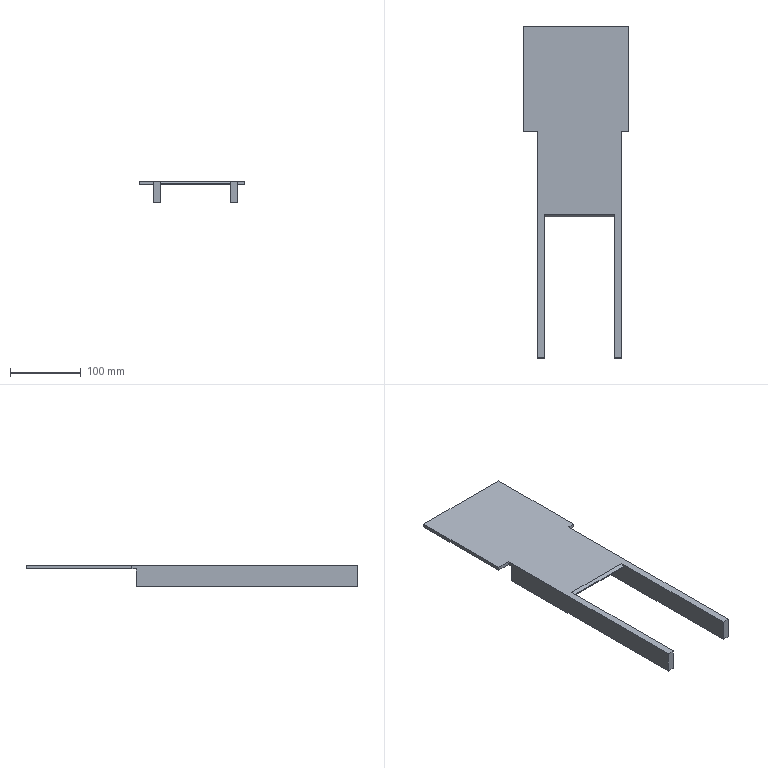Part | SolidWorks | features Chamfer 1, Extrusion 1, ICE 1 | 1 solid | 19 faces | box 150 x 470 x 30 mm | volume 353727 mm3 | plane 19
STEP:
#1=CARTESIAN_POINT('',(60.,40.,5.));
#2=VERTEX_POINT('',#1);
#3=CARTESIAN_POINT('',(60.,40.,0.));
#4=VERTEX_POINT('',#3);
#5=CARTESIAN_POINT('',(60.,40.,5.));
#6=DIRECTION('',(0.,0.,-1.));
#7=VECTOR('',#6,1000.);
#8=LINE('',#5,#7);
#9=EDGE_CURVE('',#2,#4,#8,.T.);
#10=ORIENTED_EDGE('',*,*,#9,.F.);
#11=CARTESIAN_POINT('',(60.,-280.,5.));
#12=VERTEX_POINT('',#11);
#13=CARTESIAN_POINT('',(60.,40.,5.));
#14=DIRECTION('',(0.,1.,0.));
#15=VECTOR('',#14,1000.);
#16=LINE('',#13,#15);
#17=EDGE_CURVE('',#12,#2,#16,.T.);
#18=ORIENTED_EDGE('',*,*,#17,.F.);
#19=CARTESIAN_POINT('',(60.,-280.,-25.));
#20=VERTEX_POINT('',#19);
#21=CARTESIAN_POINT('',(60.,-280.,-25.));
#22=DIRECTION('',(0.,0.,1.));
#23=VECTOR('',#22,1000.);
#24=LINE('',#21,#23);
#25=EDGE_CURVE('',#20,#12,#24,.T.);
#26=ORIENTED_EDGE('',*,*,#25,.F.);
#27=CARTESIAN_POINT('',(60.,5.758,-25.));
#28=VERTEX_POINT('',#27);
#29=CARTESIAN_POINT('',(60.,5.758,-25.));
#30=DIRECTION('',(0.,1.,0.));
#31=VECTOR('',#30,1000.);
#32=LINE('',#29,#31);
#33=EDGE_CURVE('',#20,#28,#32,.T.);
#34=ORIENTED_EDGE('',*,*,#33,.T.);
#35=CARTESIAN_POINT('',(60.,5.758,0.));
#36=VERTEX_POINT('',#35);
#37=CARTESIAN_POINT('',(60.,5.758,-25.));
#38=DIRECTION('',(0.,0.,1.));
#39=VECTOR('',#38,1000.);
#40=LINE('',#37,#39);
#41=EDGE_CURVE('',#28,#36,#40,.T.);
#42=ORIENTED_EDGE('',*,*,#41,.T.);
#43=CARTESIAN_POINT('',(60.,40.,0.));
#44=DIRECTION('',(0.,1.,0.));
#45=VECTOR('',#44,1000.);
#46=LINE('',#43,#45);
#47=EDGE_CURVE('',#36,#4,#46,.T.);
#48=ORIENTED_EDGE('',*,*,#47,.T.);
#49=EDGE_LOOP('',(#10,#18,#26,#34,#42,#48));
#50=FACE_OUTER_BOUND('',#49,.T.);
#51=CARTESIAN_POINT('',(60.,40.,5.));
#52=DIRECTION('',(-1.,0.,0.));
#53=DIRECTION('',(0.,-1.,0.));
#54=AXIS2_PLACEMENT_3D('',#51,#52,#53);
#55=PLANE('',#54);
#56=ADVANCED_FACE('',(#50),#55,.F.);
#57=CARTESIAN_POINT('',(70.,40.,0.));
#58=VERTEX_POINT('',#57);
#59=CARTESIAN_POINT('',(60.,40.,0.));
#60=DIRECTION('',(1.,0.,0.));
#61=VECTOR('',#60,1000.);
#62=LINE('',#59,#61);
#63=EDGE_CURVE('',#4,#58,#62,.T.);
#64=ORIENTED_EDGE('',*,*,#63,.T.);
#65=CARTESIAN_POINT('',(70.,40.,5.));
#66=VERTEX_POINT('',#65);
#67=CARTESIAN_POINT('',(70.,40.,5.));
#68=DIRECTION('',(0.,0.,-1.));
#69=VECTOR('',#68,1000.);
#70=LINE('',#67,#69);
#71=EDGE_CURVE('',#66,#58,#70,.T.);
#72=ORIENTED_EDGE('',*,*,#71,.F.);
#73=CARTESIAN_POINT('',(60.,40.,5.));
#74=DIRECTION('',(1.,0.,0.));
#75=VECTOR('',#74,1000.);
#76=LINE('',#73,#75);
#77=EDGE_CURVE('',#2,#66,#76,.T.);
#78=ORIENTED_EDGE('',*,*,#77,.F.);
#79=ORIENTED_EDGE('',*,*,#9,.T.);
#80=EDGE_LOOP('',(#64,#72,#78,#79));
#81=FACE_OUTER_BOUND('',#80,.T.);
#82=CARTESIAN_POINT('',(60.,40.,5.));
#83=DIRECTION('',(0.,1.,0.));
#84=DIRECTION('',(0.,0.,1.));
#85=AXIS2_PLACEMENT_3D('',#82,#83,#84);
#86=PLANE('',#85);
#87=ADVANCED_FACE('',(#81),#86,.F.);
#88=CARTESIAN_POINT('',(70.,190.,0.));
#89=VERTEX_POINT('',#88);
#90=CARTESIAN_POINT('',(70.,190.,0.));
#91=DIRECTION('',(0.,1.,0.));
#92=VECTOR('',#91,1000.);
#93=LINE('',#90,#92);
#94=EDGE_CURVE('',#58,#89,#93,.T.);
#95=ORIENTED_EDGE('',*,*,#94,.T.);
#96=CARTESIAN_POINT('',(70.,190.,5.));
#97=VERTEX_POINT('',#96);
#98=CARTESIAN_POINT('',(70.,190.,5.));
#99=DIRECTION('',(0.,0.,-1.));
#100=VECTOR('',#99,1000.);
#101=LINE('',#98,#100);
#102=EDGE_CURVE('',#97,#89,#101,.T.);
#103=ORIENTED_EDGE('',*,*,#102,.F.);
#104=CARTESIAN_POINT('',(70.,190.,5.));
#105=DIRECTION('',(0.,1.,0.));
#106=VECTOR('',#105,1000.);
#107=LINE('',#104,#106);
#108=EDGE_CURVE('',#66,#97,#107,.T.);
#109=ORIENTED_EDGE('',*,*,#108,.F.);
#110=ORIENTED_EDGE('',*,*,#71,.T.);
#111=EDGE_LOOP('',(#95,#103,#109,#110));
#112=FACE_OUTER_BOUND('',#111,.T.);
#113=CARTESIAN_POINT('',(70.,190.,5.));
#114=DIRECTION('',(-1.,0.,0.));
#115=DIRECTION('',(0.,-1.,0.));
#116=AXIS2_PLACEMENT_3D('',#113,#114,#115);
#117=PLANE('',#116);
#118=ADVANCED_FACE('',(#112),#117,.F.);
#119=CARTESIAN_POINT('',(-80.,190.,0.));
#120=VERTEX_POINT('',#119);
#121=CARTESIAN_POINT('',(-80.,190.,0.));
#122=DIRECTION('',(-1.,0.,0.));
#123=VECTOR('',#122,1000.);
#124=LINE('',#121,#123);
#125=EDGE_CURVE('',#89,#120,#124,.T.);
#126=ORIENTED_EDGE('',*,*,#125,.T.);
#127=CARTESIAN_POINT('',(-80.,190.,5.));
#128=VERTEX_POINT('',#127);
#129=CARTESIAN_POINT('',(-80.,190.,5.));
#130=DIRECTION('',(0.,0.,-1.));
#131=VECTOR('',#130,1000.);
#132=LINE('',#129,#131);
#133=EDGE_CURVE('',#128,#120,#132,.T.);
#134=ORIENTED_EDGE('',*,*,#133,.F.);
#135=CARTESIAN_POINT('',(-80.,190.,5.));
#136=DIRECTION('',(-1.,0.,0.));
#137=VECTOR('',#136,1000.);
#138=LINE('',#135,#137);
#139=EDGE_CURVE('',#97,#128,#138,.T.);
#140=ORIENTED_EDGE('',*,*,#139,.F.);
#141=ORIENTED_EDGE('',*,*,#102,.T.);
#142=EDGE_LOOP('',(#126,#134,#140,#141));
#143=FACE_OUTER_BOUND('',#142,.T.);
#144=CARTESIAN_POINT('',(-80.,190.,5.));
#145=DIRECTION('',(0.,-1.,0.));
#146=DIRECTION('',(0.,0.,-1.));
#147=AXIS2_PLACEMENT_3D('',#144,#145,#146);
#148=PLANE('',#147);
#149=ADVANCED_FACE('',(#143),#148,.F.);
#150=CARTESIAN_POINT('',(-80.,40.,0.));
#151=VERTEX_POINT('',#150);
#152=CARTESIAN_POINT('',(-80.,190.,0.));
#153=DIRECTION('',(0.,-1.,0.));
#154=VECTOR('',#153,1000.);
#155=LINE('',#152,#154);
#156=EDGE_CURVE('',#120,#151,#155,.T.);
#157=ORIENTED_EDGE('',*,*,#156,.T.);
#158=CARTESIAN_POINT('',(-80.,40.,5.));
#159=VERTEX_POINT('',#158);
#160=CARTESIAN_POINT('',(-80.,40.,5.));
#161=DIRECTION('',(0.,0.,-1.));
#162=VECTOR('',#161,1000.);
#163=LINE('',#160,#162);
#164=EDGE_CURVE('',#159,#151,#163,.T.);
#165=ORIENTED_EDGE('',*,*,#164,.F.);
#166=CARTESIAN_POINT('',(-80.,190.,5.));
#167=DIRECTION('',(0.,-1.,0.));
#168=VECTOR('',#167,1000.);
#169=LINE('',#166,#168);
#170=EDGE_CURVE('',#128,#159,#169,.T.);
#171=ORIENTED_EDGE('',*,*,#170,.F.);
#172=ORIENTED_EDGE('',*,*,#133,.T.);
#173=EDGE_LOOP('',(#157,#165,#171,#172));
#174=FACE_OUTER_BOUND('',#173,.T.);
#175=CARTESIAN_POINT('',(-80.,190.,5.));
#176=DIRECTION('',(1.,0.,0.));
#177=DIRECTION('',(0.,1.,0.));
#178=AXIS2_PLACEMENT_3D('',#175,#176,#177);
#179=PLANE('',#178);
#180=ADVANCED_FACE('',(#174),#179,.F.);
#181=CARTESIAN_POINT('',(-60.,40.,0.));
#182=VERTEX_POINT('',#181);
#183=CARTESIAN_POINT('',(-80.,40.,0.));
#184=DIRECTION('',(1.,0.,0.));
#185=VECTOR('',#184,1000.);
#186=LINE('',#183,#185);
#187=EDGE_CURVE('',#151,#182,#186,.T.);
#188=ORIENTED_EDGE('',*,*,#187,.T.);
#189=CARTESIAN_POINT('',(-60.,40.,5.));
#190=VERTEX_POINT('',#189);
#191=CARTESIAN_POINT('',(-60.,40.,5.));
#192=DIRECTION('',(0.,0.,-1.));
#193=VECTOR('',#192,1000.);
#194=LINE('',#191,#193);
#195=EDGE_CURVE('',#190,#182,#194,.T.);
#196=ORIENTED_EDGE('',*,*,#195,.F.);
#197=CARTESIAN_POINT('',(-80.,40.,5.));
#198=DIRECTION('',(1.,0.,0.));
#199=VECTOR('',#198,1000.);
#200=LINE('',#197,#199);
#201=EDGE_CURVE('',#159,#190,#200,.T.);
#202=ORIENTED_EDGE('',*,*,#201,.F.);
#203=ORIENTED_EDGE('',*,*,#164,.T.);
#204=EDGE_LOOP('',(#188,#196,#202,#203));
#205=FACE_OUTER_BOUND('',#204,.T.);
#206=CARTESIAN_POINT('',(-80.,40.,5.));
#207=DIRECTION('',(0.,1.,0.));
#208=DIRECTION('',(0.,0.,1.));
#209=AXIS2_PLACEMENT_3D('',#206,#207,#208);
#210=PLANE('',#209);
#211=ADVANCED_FACE('',(#205),#210,.F.);
#212=CARTESIAN_POINT('',(-60.,33.599,0.));
#213=VERTEX_POINT('',#212);
#214=CARTESIAN_POINT('',(-60.,40.,0.));
#215=DIRECTION('',(0.,-1.,0.));
#216=VECTOR('',#215,1000.);
#217=LINE('',#214,#216);
#218=EDGE_CURVE('',#182,#213,#217,.T.);
#219=ORIENTED_EDGE('',*,*,#218,.T.);
#220=CARTESIAN_POINT('',(-60.,33.599,-25.));
#221=VERTEX_POINT('',#220);
#222=CARTESIAN_POINT('',(-60.,33.599,-25.));
#223=DIRECTION('',(0.,0.,1.));
#224=VECTOR('',#223,1000.);
#225=LINE('',#222,#224);
#226=EDGE_CURVE('',#221,#213,#225,.T.);
#227=ORIENTED_EDGE('',*,*,#226,.F.);
#228=CARTESIAN_POINT('',(-60.,-280.,-25.));
#229=VERTEX_POINT('',#228);
#230=CARTESIAN_POINT('',(-60.,33.599,-25.));
#231=DIRECTION('',(0.,-1.,0.));
#232=VECTOR('',#231,1000.);
#233=LINE('',#230,#232);
#234=EDGE_CURVE('',#221,#229,#233,.T.);
#235=ORIENTED_EDGE('',*,*,#234,.T.);
#236=CARTESIAN_POINT('',(-60.,-280.,5.));
#237=VERTEX_POINT('',#236);
#238=CARTESIAN_POINT('',(-60.,-280.,-25.));
#239=DIRECTION('',(0.,0.,1.));
#240=VECTOR('',#239,1000.);
#241=LINE('',#238,#240);
#242=EDGE_CURVE('',#229,#237,#241,.T.);
#243=ORIENTED_EDGE('',*,*,#242,.T.);
#244=CARTESIAN_POINT('',(-60.,40.,5.));
#245=DIRECTION('',(0.,-1.,0.));
#246=VECTOR('',#245,1000.);
#247=LINE('',#244,#246);
#248=EDGE_CURVE('',#190,#237,#247,.T.);
#249=ORIENTED_EDGE('',*,*,#248,.F.);
#250=ORIENTED_EDGE('',*,*,#195,.T.);
#251=EDGE_LOOP('',(#219,#227,#235,#243,#249,#250));
#252=FACE_OUTER_BOUND('',#251,.T.);
#253=CARTESIAN_POINT('',(-60.,40.,5.));
#254=DIRECTION('',(1.,0.,0.));
#255=DIRECTION('',(0.,1.,0.));
#256=AXIS2_PLACEMENT_3D('',#253,#254,#255);
#257=PLANE('',#256);
#258=ADVANCED_FACE('',(#252),#257,.F.);
#259=CARTESIAN_POINT('',(50.,-80.,0.));
#260=VERTEX_POINT('',#259);
#261=CARTESIAN_POINT('',(50.,-80.,1.5));
#262=VERTEX_POINT('',#261);
#263=CARTESIAN_POINT('',(50.,-80.,5.));
#264=DIRECTION('',(0.,0.,1.));
#265=VECTOR('',#264,1000.);
#266=LINE('',#263,#265);
#267=EDGE_CURVE('',#260,#262,#266,.T.);
#268=ORIENTED_EDGE('',*,*,#267,.T.);
#269=CARTESIAN_POINT('',(-50.,-80.,1.5));
#270=VERTEX_POINT('',#269);
#271=CARTESIAN_POINT('',(-50.,-80.,1.5));
#272=DIRECTION('',(-1.,0.,0.));
#273=VECTOR('',#272,1000.);
#274=LINE('',#271,#273);
#275=EDGE_CURVE('',#262,#270,#274,.T.);
#276=ORIENTED_EDGE('',*,*,#275,.T.);
#277=CARTESIAN_POINT('',(-50.,-80.,0.));
#278=VERTEX_POINT('',#277);
#279=CARTESIAN_POINT('',(-50.,-80.,5.));
#280=DIRECTION('',(0.,0.,-1.));
#281=VECTOR('',#280,1000.);
#282=LINE('',#279,#281);
#283=EDGE_CURVE('',#270,#278,#282,.T.);
#284=ORIENTED_EDGE('',*,*,#283,.T.);
#285=CARTESIAN_POINT('',(-60.,-80.,0.));
#286=DIRECTION('',(1.,0.,0.));
#287=VECTOR('',#286,1000.);
#288=LINE('',#285,#287);
#289=EDGE_CURVE('',#278,#260,#288,.T.);
#290=ORIENTED_EDGE('',*,*,#289,.T.);
#291=EDGE_LOOP('',(#268,#276,#284,#290));
#292=FACE_OUTER_BOUND('',#291,.T.);
#293=CARTESIAN_POINT('',(-60.,-80.,5.));
#294=DIRECTION('',(0.,1.,0.));
#295=DIRECTION('',(0.,0.,1.));
#296=AXIS2_PLACEMENT_3D('',#293,#294,#295);
#297=PLANE('',#296);
#298=ADVANCED_FACE('',(#292),#297,.F.);
#299=CARTESIAN_POINT('',(-50.,-76.5,5.));
#300=VERTEX_POINT('',#299);
#301=CARTESIAN_POINT('',(50.,-76.5,5.));
#302=VERTEX_POINT('',#301);
#303=CARTESIAN_POINT('',(50.,-76.5,5.));
#304=DIRECTION('',(1.,0.,0.));
#305=VECTOR('',#304,1000.);
#306=LINE('',#303,#305);
#307=EDGE_CURVE('',#300,#302,#306,.T.);
#308=ORIENTED_EDGE('',*,*,#307,.T.);
#309=CARTESIAN_POINT('',(50.,-280.,5.));
#310=VERTEX_POINT('',#309);
#311=CARTESIAN_POINT('',(50.,5.758,5.));
#312=DIRECTION('',(0.,-1.,0.));
#313=VECTOR('',#312,1000.);
#314=LINE('',#311,#313);
#315=EDGE_CURVE('',#302,#310,#314,.T.);
#316=ORIENTED_EDGE('',*,*,#315,.T.);
#317=CARTESIAN_POINT('',(60.,-280.,5.));
#318=DIRECTION('',(1.,0.,0.));
#319=VECTOR('',#318,1000.);
#320=LINE('',#317,#319);
#321=EDGE_CURVE('',#310,#12,#320,.T.);
#322=ORIENTED_EDGE('',*,*,#321,.T.);
#323=ORIENTED_EDGE('',*,*,#17,.T.);
#324=ORIENTED_EDGE('',*,*,#77,.T.);
#325=ORIENTED_EDGE('',*,*,#108,.T.);
#326=ORIENTED_EDGE('',*,*,#139,.T.);
#327=ORIENTED_EDGE('',*,*,#170,.T.);
#328=ORIENTED_EDGE('',*,*,#201,.T.);
#329=ORIENTED_EDGE('',*,*,#248,.T.);
#330=CARTESIAN_POINT('',(-50.,-280.,5.));
#331=VERTEX_POINT('',#330);
#332=CARTESIAN_POINT('',(-60.,-280.,5.));
#333=DIRECTION('',(1.,0.,0.));
#334=VECTOR('',#333,1000.);
#335=LINE('',#332,#334);
#336=EDGE_CURVE('',#237,#331,#335,.T.);
#337=ORIENTED_EDGE('',*,*,#336,.T.);
#338=CARTESIAN_POINT('',(-50.,33.599,5.));
#339=DIRECTION('',(0.,1.,0.));
#340=VECTOR('',#339,1000.);
#341=LINE('',#338,#340);
#342=EDGE_CURVE('',#331,#300,#341,.T.);
#343=ORIENTED_EDGE('',*,*,#342,.T.);
#344=EDGE_LOOP('',(#308,#316,#322,#323,#324,#325,#326,#327,#328,#329,#337,#343));
#345=FACE_OUTER_BOUND('',#344,.T.);
#346=CARTESIAN_POINT('',(0.,0.,5.));
#347=DIRECTION('',(0.,0.,1.));
#348=DIRECTION('',(1.,0.,0.));
#349=AXIS2_PLACEMENT_3D('',#346,#347,#348);
#350=PLANE('',#349);
#351=ADVANCED_FACE('',(#345),#350,.T.);
#352=CARTESIAN_POINT('',(-50.,33.599,0.));
#353=VERTEX_POINT('',#352);
#354=CARTESIAN_POINT('',(-50.,0.,0.));
#355=DIRECTION('',(0.,1.,0.));
#356=VECTOR('',#355,1000.);
#357=LINE('',#354,#356);
#358=EDGE_CURVE('',#278,#353,#357,.T.);
#359=ORIENTED_EDGE('',*,*,#358,.T.);
#360=CARTESIAN_POINT('',(0.,33.599,0.));
#361=DIRECTION('',(-1.,0.,0.));
#362=VECTOR('',#361,1000.);
#363=LINE('',#360,#362);
#364=EDGE_CURVE('',#353,#213,#363,.T.);
#365=ORIENTED_EDGE('',*,*,#364,.T.);
#366=ORIENTED_EDGE('',*,*,#218,.F.);
#367=ORIENTED_EDGE('',*,*,#187,.F.);
#368=ORIENTED_EDGE('',*,*,#156,.F.);
#369=ORIENTED_EDGE('',*,*,#125,.F.);
#370=ORIENTED_EDGE('',*,*,#94,.F.);
#371=ORIENTED_EDGE('',*,*,#63,.F.);
#372=ORIENTED_EDGE('',*,*,#47,.F.);
#373=CARTESIAN_POINT('',(50.,5.758,0.));
#374=VERTEX_POINT('',#373);
#375=CARTESIAN_POINT('',(0.,5.758,0.));
#376=DIRECTION('',(-1.,0.,0.));
#377=VECTOR('',#376,1000.);
#378=LINE('',#375,#377);
#379=EDGE_CURVE('',#36,#374,#378,.T.);
#380=ORIENTED_EDGE('',*,*,#379,.T.);
#381=CARTESIAN_POINT('',(50.,0.,0.));
#382=DIRECTION('',(0.,-1.,0.));
#383=VECTOR('',#382,1000.);
#384=LINE('',#381,#383);
#385=EDGE_CURVE('',#374,#260,#384,.T.);
#386=ORIENTED_EDGE('',*,*,#385,.T.);
#387=ORIENTED_EDGE('',*,*,#289,.F.);
#388=EDGE_LOOP('',(#359,#365,#366,#367,#368,#369,#370,#371,#372,#380,#386,#387));
#389=FACE_OUTER_BOUND('',#388,.T.);
#390=CARTESIAN_POINT('',(0.,0.,0.));
#391=DIRECTION('',(0.,0.,1.));
#392=DIRECTION('',(1.,0.,0.));
#393=AXIS2_PLACEMENT_3D('',#390,#391,#392);
#394=PLANE('',#393);
#395=ADVANCED_FACE('',(#389),#394,.F.);
#396=ORIENTED_EDGE('',*,*,#267,.F.);
#397=ORIENTED_EDGE('',*,*,#385,.F.);
#398=CARTESIAN_POINT('',(50.,5.758,-25.));
#399=VERTEX_POINT('',#398);
#400=CARTESIAN_POINT('',(50.,5.758,-25.));
#401=DIRECTION('',(0.,0.,1.));
#402=VECTOR('',#401,1000.);
#403=LINE('',#400,#402);
#404=EDGE_CURVE('',#399,#374,#403,.T.);
#405=ORIENTED_EDGE('',*,*,#404,.F.);
#406=CARTESIAN_POINT('',(50.,-280.,-25.));
#407=VERTEX_POINT('',#406);
#408=CARTESIAN_POINT('',(50.,5.758,-25.));
#409=DIRECTION('',(0.,-1.,0.));
#410=VECTOR('',#409,1000.);
#411=LINE('',#408,#410);
#412=EDGE_CURVE('',#399,#407,#411,.T.);
#413=ORIENTED_EDGE('',*,*,#412,.T.);
#414=CARTESIAN_POINT('',(50.,-280.,-25.));
#415=DIRECTION('',(0.,0.,1.));
#416=VECTOR('',#415,1000.);
#417=LINE('',#414,#416);
#418=EDGE_CURVE('',#407,#310,#417,.T.);
#419=ORIENTED_EDGE('',*,*,#418,.T.);
#420=ORIENTED_EDGE('',*,*,#315,.F.);
#421=CARTESIAN_POINT('',(50.,-76.5,5.));
#422=DIRECTION('',(0.,-0.7071,-0.7071));
#423=VECTOR('',#422,1000.);
#424=LINE('',#421,#423);
#425=EDGE_CURVE('',#302,#262,#424,.T.);
#426=ORIENTED_EDGE('',*,*,#425,.T.);
#427=EDGE_LOOP('',(#396,#397,#405,#413,#419,#420,#426));
#428=FACE_OUTER_BOUND('',#427,.T.);
#429=CARTESIAN_POINT('',(50.,5.758,-25.));
#430=DIRECTION('',(-1.,0.,0.));
#431=DIRECTION('',(0.,-1.,0.));
#432=AXIS2_PLACEMENT_3D('',#429,#430,#431);
#433=PLANE('',#432);
#434=ADVANCED_FACE('',(#428),#433,.T.);
#435=ORIENTED_EDGE('',*,*,#379,.F.);
#436=ORIENTED_EDGE('',*,*,#41,.F.);
#437=CARTESIAN_POINT('',(60.,5.758,-25.));
#438=DIRECTION('',(-1.,0.,0.));
#439=VECTOR('',#438,1000.);
#440=LINE('',#437,#439);
#441=EDGE_CURVE('',#28,#399,#440,.T.);
#442=ORIENTED_EDGE('',*,*,#441,.T.);
#443=ORIENTED_EDGE('',*,*,#404,.T.);
#444=EDGE_LOOP('',(#435,#436,#442,#443));
#445=FACE_OUTER_BOUND('',#444,.T.);
#446=CARTESIAN_POINT('',(60.,5.758,-25.));
#447=DIRECTION('',(0.,1.,0.));
#448=DIRECTION('',(-1.,0.,0.));
#449=AXIS2_PLACEMENT_3D('',#446,#447,#448);
#450=PLANE('',#449);
#451=ADVANCED_FACE('',(#445),#450,.T.);
#452=ORIENTED_EDGE('',*,*,#321,.F.);
#453=ORIENTED_EDGE('',*,*,#418,.F.);
#454=CARTESIAN_POINT('',(60.,-280.,-25.));
#455=DIRECTION('',(1.,0.,0.));
#456=VECTOR('',#455,1000.);
#457=LINE('',#454,#456);
#458=EDGE_CURVE('',#407,#20,#457,.T.);
#459=ORIENTED_EDGE('',*,*,#458,.T.);
#460=ORIENTED_EDGE('',*,*,#25,.T.);
#461=EDGE_LOOP('',(#452,#453,#459,#460));
#462=FACE_OUTER_BOUND('',#461,.T.);
#463=CARTESIAN_POINT('',(60.,-280.,-25.));
#464=DIRECTION('',(0.,-1.,0.));
#465=DIRECTION('',(0.,0.,-1.));
#466=AXIS2_PLACEMENT_3D('',#463,#464,#465);
#467=PLANE('',#466);
#468=ADVANCED_FACE('',(#462),#467,.T.);
#469=ORIENTED_EDGE('',*,*,#33,.F.);
#470=ORIENTED_EDGE('',*,*,#458,.F.);
#471=ORIENTED_EDGE('',*,*,#412,.F.);
#472=ORIENTED_EDGE('',*,*,#441,.F.);
#473=EDGE_LOOP('',(#469,#470,#471,#472));
#474=FACE_OUTER_BOUND('',#473,.T.);
#475=CARTESIAN_POINT('',(0.,0.,-25.));
#476=DIRECTION('',(0.,0.,-1.));
#477=DIRECTION('',(-1.,0.,0.));
#478=AXIS2_PLACEMENT_3D('',#475,#476,#477);
#479=PLANE('',#478);
#480=ADVANCED_FACE('',(#474),#479,.T.);
#481=ORIENTED_EDGE('',*,*,#364,.F.);
#482=CARTESIAN_POINT('',(-50.,33.599,-25.));
#483=VERTEX_POINT('',#482);
#484=CARTESIAN_POINT('',(-50.,33.599,-25.));
#485=DIRECTION('',(0.,0.,1.));
#486=VECTOR('',#485,1000.);
#487=LINE('',#484,#486);
#488=EDGE_CURVE('',#483,#353,#487,.T.);
#489=ORIENTED_EDGE('',*,*,#488,.F.);
#490=CARTESIAN_POINT('',(-60.,33.599,-25.));
#491=DIRECTION('',(-1.,0.,0.));
#492=VECTOR('',#491,1000.);
#493=LINE('',#490,#492);
#494=EDGE_CURVE('',#483,#221,#493,.T.);
#495=ORIENTED_EDGE('',*,*,#494,.T.);
#496=ORIENTED_EDGE('',*,*,#226,.T.);
#497=EDGE_LOOP('',(#481,#489,#495,#496));
#498=FACE_OUTER_BOUND('',#497,.T.);
#499=CARTESIAN_POINT('',(-60.,33.599,-25.));
#500=DIRECTION('',(0.,1.,0.));
#501=DIRECTION('',(0.,0.,1.));
#502=AXIS2_PLACEMENT_3D('',#499,#500,#501);
#503=PLANE('',#502);
#504=ADVANCED_FACE('',(#498),#503,.T.);
#505=ORIENTED_EDGE('',*,*,#283,.F.);
#506=CARTESIAN_POINT('',(-50.,-76.5,5.));
#507=DIRECTION('',(0.,0.7071,0.7071));
#508=VECTOR('',#507,1000.);
#509=LINE('',#506,#508);
#510=EDGE_CURVE('',#270,#300,#509,.T.);
#511=ORIENTED_EDGE('',*,*,#510,.T.);
#512=ORIENTED_EDGE('',*,*,#342,.F.);
#513=CARTESIAN_POINT('',(-50.,-280.,-25.));
#514=VERTEX_POINT('',#513);
#515=CARTESIAN_POINT('',(-50.,-280.,-25.));
#516=DIRECTION('',(0.,0.,1.));
#517=VECTOR('',#516,1000.);
#518=LINE('',#515,#517);
#519=EDGE_CURVE('',#514,#331,#518,.T.);
#520=ORIENTED_EDGE('',*,*,#519,.F.);
#521=CARTESIAN_POINT('',(-50.,33.599,-25.));
#522=DIRECTION('',(0.,1.,0.));
#523=VECTOR('',#522,1000.);
#524=LINE('',#521,#523);
#525=EDGE_CURVE('',#514,#483,#524,.T.);
#526=ORIENTED_EDGE('',*,*,#525,.T.);
#527=ORIENTED_EDGE('',*,*,#488,.T.);
#528=ORIENTED_EDGE('',*,*,#358,.F.);
#529=EDGE_LOOP('',(#505,#511,#512,#520,#526,#527,#528));
#530=FACE_OUTER_BOUND('',#529,.T.);
#531=CARTESIAN_POINT('',(-50.,33.599,-25.));
#532=DIRECTION('',(1.,0.,0.));
#533=DIRECTION('',(0.,1.,0.));
#534=AXIS2_PLACEMENT_3D('',#531,#532,#533);
#535=PLANE('',#534);
#536=ADVANCED_FACE('',(#530),#535,.T.);
#537=ORIENTED_EDGE('',*,*,#336,.F.);
#538=ORIENTED_EDGE('',*,*,#242,.F.);
#539=CARTESIAN_POINT('',(-60.,-280.,-25.));
#540=DIRECTION('',(1.,0.,0.));
#541=VECTOR('',#540,1000.);
#542=LINE('',#539,#541);
#543=EDGE_CURVE('',#229,#514,#542,.T.);
#544=ORIENTED_EDGE('',*,*,#543,.T.);
#545=ORIENTED_EDGE('',*,*,#519,.T.);
#546=EDGE_LOOP('',(#537,#538,#544,#545));
#547=FACE_OUTER_BOUND('',#546,.T.);
#548=CARTESIAN_POINT('',(-60.,-280.,-25.));
#549=DIRECTION('',(0.,-1.,0.));
#550=DIRECTION('',(0.,0.,-1.));
#551=AXIS2_PLACEMENT_3D('',#548,#549,#550);
#552=PLANE('',#551);
#553=ADVANCED_FACE('',(#547),#552,.T.);
#554=ORIENTED_EDGE('',*,*,#234,.F.);
#555=ORIENTED_EDGE('',*,*,#494,.F.);
#556=ORIENTED_EDGE('',*,*,#525,.F.);
#557=ORIENTED_EDGE('',*,*,#543,.F.);
#558=EDGE_LOOP('',(#554,#555,#556,#557));
#559=FACE_OUTER_BOUND('',#558,.T.);
#560=CARTESIAN_POINT('',(0.,0.,-25.));
#561=DIRECTION('',(0.,0.,1.));
#562=DIRECTION('',(1.,0.,0.));
#563=AXIS2_PLACEMENT_3D('',#560,#561,#562);
#564=PLANE('',#563);
#565=ADVANCED_FACE('',(#559),#564,.F.);
#566=ORIENTED_EDGE('',*,*,#510,.F.);
#567=ORIENTED_EDGE('',*,*,#275,.F.);
#568=ORIENTED_EDGE('',*,*,#425,.F.);
#569=ORIENTED_EDGE('',*,*,#307,.F.);
#570=EDGE_LOOP('',(#566,#567,#568,#569));
#571=FACE_OUTER_BOUND('',#570,.T.);
#572=CARTESIAN_POINT('',(0.,-76.5,5.));
#573=DIRECTION('',(0.,-0.7071,0.7071));
#574=DIRECTION('',(-1.,0.,0.));
#575=AXIS2_PLACEMENT_3D('',#572,#573,#574);
#576=PLANE('',#575);
#577=ADVANCED_FACE('',(#571),#576,.T.);
#578=CLOSED_SHELL('',(#56,#87,#118,#149,#180,#211,#258,#298,#351,#395,#434,#451,#468,#480,#504,#536,#553,#565,#577));
#579=MANIFOLD_SOLID_BREP('',#578);
#580=CARTESIAN_POINT('',(0.,0.,0.));
#581=DIRECTION('',(0.,0.,1.));
#582=DIRECTION('',(1.,0.,0.));
#583=AXIS2_PLACEMENT_3D('',#580,#581,#582);
#584=(LENGTH_UNIT()NAMED_UNIT(*)SI_UNIT(.MILLI.,.METRE.));
#585=UNCERTAINTY_MEASURE_WITH_UNIT(LENGTH_MEASURE(0.00001),#584,'','');
#586=(NAMED_UNIT(*)PLANE_ANGLE_UNIT()SI_UNIT($,.RADIAN.));
#587=(NAMED_UNIT(*)SI_UNIT($,.STERADIAN.)SOLID_ANGLE_UNIT());
#588=(GEOMETRIC_REPRESENTATION_CONTEXT(3)GLOBAL_UNCERTAINTY_ASSIGNED_CONTEXT((#585))GLOBAL_UNIT_ASSIGNED_CONTEXT((#584,#586,#587))REPRESENTATION_CONTEXT('',''));
#589=ADVANCED_BREP_SHAPE_REPRESENTATION('',(#579,#583),#588);